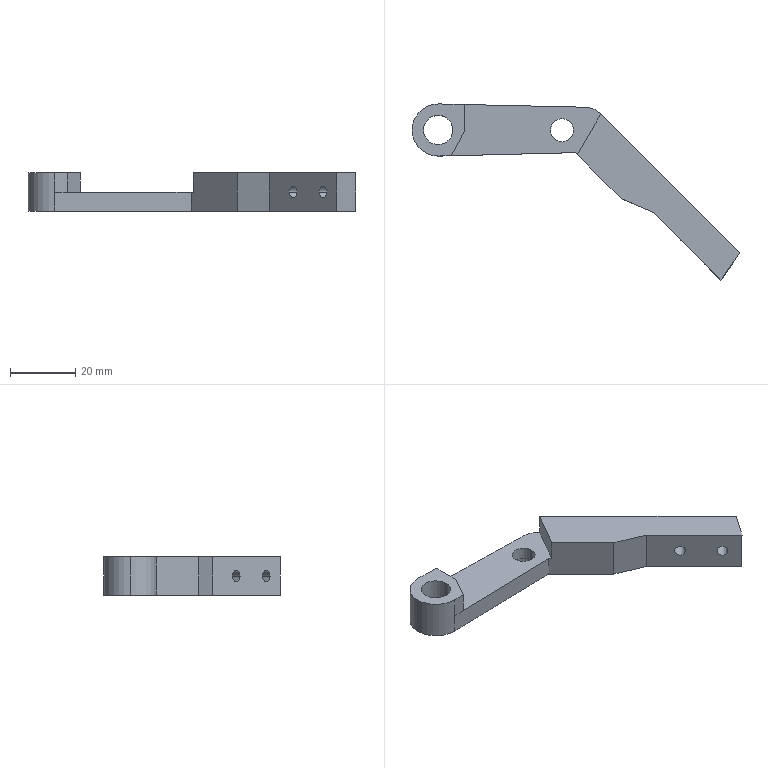Part | STEP file | Ngam kep 3 | 1 solid | 30 faces | box 100.617 x 54.035 x 11.8 mm | volume 12936 mm3 | plane 17 | cylinder 13 | commonest cylinder face diameters 3.3 x4 9 x4 7 x2 16 x2 14 x1